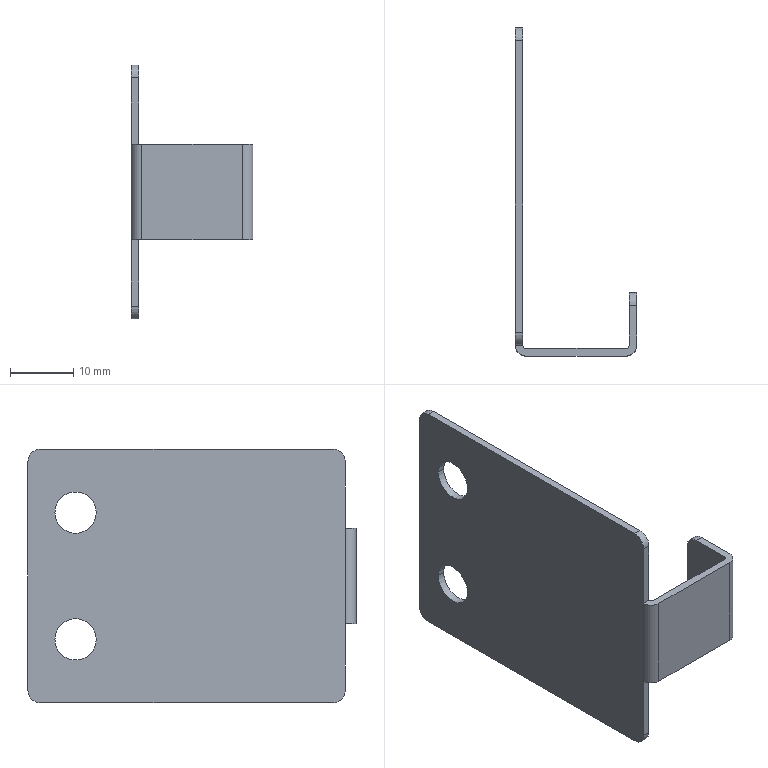Part | SolidWorks | features BaseBody 1 | 1 solid | 28 faces | box 19.2 x 51.7 x 40 mm | volume 2810 mm3 | cylinder 14 | plane 14 | commonest cylinder face diameters 4 x6 6.5 x4 1 x2 3.4 x2
STEP:
#1=CARTESIAN_POINT('',(-1.2,45.75,30.));
#2=VERTEX_POINT('',#1);
#3=CARTESIAN_POINT('',(-1.2,39.25,30.));
#4=VERTEX_POINT('',#3);
#5=CARTESIAN_POINT('',(-1.2,42.5,30.));
#6=DIRECTION('',(-1.,0.,0.));
#7=DIRECTION('',(0.,1.,0.));
#8=AXIS2_PLACEMENT_3D('',#5,#6,#7);
#9=CIRCLE('',#8,3.25);
#10=EDGE_CURVE('',#2,#4,#9,.T.);
#11=ORIENTED_EDGE('',*,*,#10,.T.);
#12=CARTESIAN_POINT('',(0.,39.25,30.));
#13=VERTEX_POINT('',#12);
#14=CARTESIAN_POINT('',(-10.,39.25,30.));
#15=DIRECTION('',(1.,0.,0.));
#16=VECTOR('',#15,1000.);
#17=LINE('',#14,#16);
#18=EDGE_CURVE('',#4,#13,#17,.T.);
#19=ORIENTED_EDGE('',*,*,#18,.T.);
#20=CARTESIAN_POINT('',(0.,45.75,30.));
#21=VERTEX_POINT('',#20);
#22=CARTESIAN_POINT('',(0.,42.5,30.));
#23=DIRECTION('',(-1.,0.,0.));
#24=DIRECTION('',(0.,1.,0.));
#25=AXIS2_PLACEMENT_3D('',#22,#23,#24);
#26=CIRCLE('',#25,3.25);
#27=EDGE_CURVE('',#21,#13,#26,.T.);
#28=ORIENTED_EDGE('',*,*,#27,.F.);
#29=CARTESIAN_POINT('',(-10.,45.75,30.));
#30=DIRECTION('',(1.,0.,0.));
#31=VECTOR('',#30,1000.);
#32=LINE('',#29,#31);
#33=EDGE_CURVE('',#2,#21,#32,.T.);
#34=ORIENTED_EDGE('',*,*,#33,.F.);
#35=EDGE_LOOP('',(#11,#19,#28,#34));
#36=FACE_OUTER_BOUND('',#35,.T.);
#37=CARTESIAN_POINT('',(-10.,42.5,30.));
#38=DIRECTION('',(1.,0.,0.));
#39=DIRECTION('',(0.,1.,0.));
#40=AXIS2_PLACEMENT_3D('',#37,#38,#39);
#41=CYLINDRICAL_SURFACE('',#40,3.25);
#42=ADVANCED_FACE('',(#36),#41,.F.);
#43=CARTESIAN_POINT('',(-1.2,45.75,10.));
#44=VERTEX_POINT('',#43);
#45=CARTESIAN_POINT('',(-1.2,39.25,10.));
#46=VERTEX_POINT('',#45);
#47=CARTESIAN_POINT('',(-1.2,42.5,10.));
#48=DIRECTION('',(-1.,0.,0.));
#49=DIRECTION('',(0.,1.,0.));
#50=AXIS2_PLACEMENT_3D('',#47,#48,#49);
#51=CIRCLE('',#50,3.25);
#52=EDGE_CURVE('',#44,#46,#51,.T.);
#53=ORIENTED_EDGE('',*,*,#52,.T.);
#54=CARTESIAN_POINT('',(0.,39.25,10.));
#55=VERTEX_POINT('',#54);
#56=CARTESIAN_POINT('',(-10.,39.25,10.));
#57=DIRECTION('',(1.,0.,0.));
#58=VECTOR('',#57,1000.);
#59=LINE('',#56,#58);
#60=EDGE_CURVE('',#46,#55,#59,.T.);
#61=ORIENTED_EDGE('',*,*,#60,.T.);
#62=CARTESIAN_POINT('',(0.,45.75,10.));
#63=VERTEX_POINT('',#62);
#64=CARTESIAN_POINT('',(0.,42.5,10.));
#65=DIRECTION('',(-1.,0.,0.));
#66=DIRECTION('',(0.,1.,0.));
#67=AXIS2_PLACEMENT_3D('',#64,#65,#66);
#68=CIRCLE('',#67,3.25);
#69=EDGE_CURVE('',#63,#55,#68,.T.);
#70=ORIENTED_EDGE('',*,*,#69,.F.);
#71=CARTESIAN_POINT('',(-10.,45.75,10.));
#72=DIRECTION('',(1.,0.,0.));
#73=VECTOR('',#72,1000.);
#74=LINE('',#71,#73);
#75=EDGE_CURVE('',#44,#63,#74,.T.);
#76=ORIENTED_EDGE('',*,*,#75,.F.);
#77=EDGE_LOOP('',(#53,#61,#70,#76));
#78=FACE_OUTER_BOUND('',#77,.T.);
#79=CARTESIAN_POINT('',(-10.,42.5,10.));
#80=DIRECTION('',(1.,0.,0.));
#81=DIRECTION('',(0.,1.,0.));
#82=AXIS2_PLACEMENT_3D('',#79,#80,#81);
#83=CYLINDRICAL_SURFACE('',#82,3.25);
#84=ADVANCED_FACE('',(#78),#83,.F.);
#85=CARTESIAN_POINT('',(-1.2,48.,0.));
#86=VERTEX_POINT('',#85);
#87=CARTESIAN_POINT('',(-1.2,50.,2.));
#88=VERTEX_POINT('',#87);
#89=CARTESIAN_POINT('',(-1.2,48.,2.));
#90=DIRECTION('',(1.,0.,0.));
#91=DIRECTION('',(0.,0.,-1.));
#92=AXIS2_PLACEMENT_3D('',#89,#90,#91);
#93=CIRCLE('',#92,2.);
#94=EDGE_CURVE('',#86,#88,#93,.T.);
#95=ORIENTED_EDGE('',*,*,#94,.F.);
#96=CARTESIAN_POINT('',(-1.2,2.,0.));
#97=VERTEX_POINT('',#96);
#98=CARTESIAN_POINT('',(-1.2,50.,0.));
#99=DIRECTION('',(0.,1.,0.));
#100=VECTOR('',#99,1000.);
#101=LINE('',#98,#100);
#102=EDGE_CURVE('',#97,#86,#101,.T.);
#103=ORIENTED_EDGE('',*,*,#102,.F.);
#104=CARTESIAN_POINT('',(-1.2,0.,2.));
#105=VERTEX_POINT('',#104);
#106=CARTESIAN_POINT('',(-1.2,2.,2.));
#107=DIRECTION('',(1.,0.,0.));
#108=DIRECTION('',(0.,0.,1.));
#109=AXIS2_PLACEMENT_3D('',#106,#107,#108);
#110=CIRCLE('',#109,2.);
#111=EDGE_CURVE('',#105,#97,#110,.T.);
#112=ORIENTED_EDGE('',*,*,#111,.F.);
#113=CARTESIAN_POINT('',(-1.2,0.,12.5));
#114=VERTEX_POINT('',#113);
#115=CARTESIAN_POINT('',(-1.2,0.,40.));
#116=DIRECTION('',(0.,0.,-1.));
#117=VECTOR('',#116,1000.);
#118=LINE('',#115,#117);
#119=EDGE_CURVE('',#114,#105,#118,.T.);
#120=ORIENTED_EDGE('',*,*,#119,.F.);
#121=CARTESIAN_POINT('',(-1.2,0.,27.5));
#122=VERTEX_POINT('',#121);
#123=CARTESIAN_POINT('',(-1.2,0.,40.));
#124=DIRECTION('',(0.,0.,-1.));
#125=VECTOR('',#124,1000.);
#126=LINE('',#123,#125);
#127=EDGE_CURVE('',#122,#114,#126,.T.);
#128=ORIENTED_EDGE('',*,*,#127,.F.);
#129=CARTESIAN_POINT('',(-1.2,0.,38.));
#130=VERTEX_POINT('',#129);
#131=CARTESIAN_POINT('',(-1.2,0.,40.));
#132=DIRECTION('',(0.,0.,-1.));
#133=VECTOR('',#132,1000.);
#134=LINE('',#131,#133);
#135=EDGE_CURVE('',#130,#122,#134,.T.);
#136=ORIENTED_EDGE('',*,*,#135,.F.);
#137=CARTESIAN_POINT('',(-1.2,2.,40.));
#138=VERTEX_POINT('',#137);
#139=CARTESIAN_POINT('',(-1.2,2.,38.));
#140=DIRECTION('',(1.,0.,0.));
#141=DIRECTION('',(0.,0.,-1.));
#142=AXIS2_PLACEMENT_3D('',#139,#140,#141);
#143=CIRCLE('',#142,2.);
#144=EDGE_CURVE('',#138,#130,#143,.T.);
#145=ORIENTED_EDGE('',*,*,#144,.F.);
#146=CARTESIAN_POINT('',(-1.2,48.,40.));
#147=VERTEX_POINT('',#146);
#148=CARTESIAN_POINT('',(-1.2,50.,40.));
#149=DIRECTION('',(0.,-1.,0.));
#150=VECTOR('',#149,1000.);
#151=LINE('',#148,#150);
#152=EDGE_CURVE('',#147,#138,#151,.T.);
#153=ORIENTED_EDGE('',*,*,#152,.F.);
#154=CARTESIAN_POINT('',(-1.2,50.,38.));
#155=VERTEX_POINT('',#154);
#156=CARTESIAN_POINT('',(-1.2,48.,38.));
#157=DIRECTION('',(1.,0.,0.));
#158=DIRECTION('',(0.,0.,1.));
#159=AXIS2_PLACEMENT_3D('',#156,#157,#158);
#160=CIRCLE('',#159,2.);
#161=EDGE_CURVE('',#155,#147,#160,.T.);
#162=ORIENTED_EDGE('',*,*,#161,.F.);
#163=CARTESIAN_POINT('',(-1.2,50.,40.));
#164=DIRECTION('',(0.,0.,1.));
#165=VECTOR('',#164,1000.);
#166=LINE('',#163,#165);
#167=EDGE_CURVE('',#88,#155,#166,.T.);
#168=ORIENTED_EDGE('',*,*,#167,.F.);
#169=EDGE_LOOP('',(#95,#103,#112,#120,#128,#136,#145,#153,#162,#168));
#170=FACE_OUTER_BOUND('',#169,.T.);
#171=ORIENTED_EDGE('',*,*,#10,.F.);
#172=CARTESIAN_POINT('',(-1.2,42.5,30.));
#173=DIRECTION('',(-1.,0.,0.));
#174=DIRECTION('',(0.,1.,0.));
#175=AXIS2_PLACEMENT_3D('',#172,#173,#174);
#176=CIRCLE('',#175,3.25);
#177=EDGE_CURVE('',#4,#2,#176,.T.);
#178=ORIENTED_EDGE('',*,*,#177,.F.);
#179=EDGE_LOOP('',(#171,#178));
#180=FACE_BOUND('',#179,.T.);
#181=ORIENTED_EDGE('',*,*,#52,.F.);
#182=CARTESIAN_POINT('',(-1.2,42.5,10.));
#183=DIRECTION('',(-1.,0.,0.));
#184=DIRECTION('',(0.,1.,0.));
#185=AXIS2_PLACEMENT_3D('',#182,#183,#184);
#186=CIRCLE('',#185,3.25);
#187=EDGE_CURVE('',#46,#44,#186,.T.);
#188=ORIENTED_EDGE('',*,*,#187,.F.);
#189=EDGE_LOOP('',(#181,#188));
#190=FACE_BOUND('',#189,.T.);
#191=CARTESIAN_POINT('',(-1.2,50.,40.));
#192=DIRECTION('',(1.,0.,0.));
#193=DIRECTION('',(0.,1.,0.));
#194=AXIS2_PLACEMENT_3D('',#191,#192,#193);
#195=PLANE('',#194);
#196=ADVANCED_FACE('',(#170,#180,#190),#195,.F.);
#197=ORIENTED_EDGE('',*,*,#167,.T.);
#198=CARTESIAN_POINT('',(0.,50.,38.));
#199=VERTEX_POINT('',#198);
#200=CARTESIAN_POINT('',(-1.2,50.,38.));
#201=DIRECTION('',(1.,0.,0.));
#202=VECTOR('',#201,1000.);
#203=LINE('',#200,#202);
#204=EDGE_CURVE('',#155,#199,#203,.T.);
#205=ORIENTED_EDGE('',*,*,#204,.T.);
#206=CARTESIAN_POINT('',(0.,50.,2.));
#207=VERTEX_POINT('',#206);
#208=CARTESIAN_POINT('',(0.,50.,40.));
#209=DIRECTION('',(0.,0.,-1.));
#210=VECTOR('',#209,1000.);
#211=LINE('',#208,#210);
#212=EDGE_CURVE('',#199,#207,#211,.T.);
#213=ORIENTED_EDGE('',*,*,#212,.T.);
#214=CARTESIAN_POINT('',(-1.2,50.,2.));
#215=DIRECTION('',(-1.,0.,0.));
#216=VECTOR('',#215,1000.);
#217=LINE('',#214,#216);
#218=EDGE_CURVE('',#207,#88,#217,.T.);
#219=ORIENTED_EDGE('',*,*,#218,.T.);
#220=EDGE_LOOP('',(#197,#205,#213,#219));
#221=FACE_OUTER_BOUND('',#220,.T.);
#222=CARTESIAN_POINT('',(-1.2,50.,40.));
#223=DIRECTION('',(0.,1.,0.));
#224=DIRECTION('',(0.,0.,1.));
#225=AXIS2_PLACEMENT_3D('',#222,#223,#224);
#226=PLANE('',#225);
#227=ADVANCED_FACE('',(#221),#226,.T.);
#228=CARTESIAN_POINT('',(0.,48.,0.));
#229=VERTEX_POINT('',#228);
#230=CARTESIAN_POINT('',(0.,48.,2.));
#231=DIRECTION('',(-1.,0.,0.));
#232=DIRECTION('',(0.,0.,-1.));
#233=AXIS2_PLACEMENT_3D('',#230,#231,#232);
#234=CIRCLE('',#233,2.);
#235=EDGE_CURVE('',#207,#229,#234,.T.);
#236=ORIENTED_EDGE('',*,*,#235,.T.);
#237=CARTESIAN_POINT('',(0.,48.,0.));
#238=DIRECTION('',(-1.,0.,0.));
#239=VECTOR('',#238,1000.);
#240=LINE('',#237,#239);
#241=EDGE_CURVE('',#229,#86,#240,.T.);
#242=ORIENTED_EDGE('',*,*,#241,.T.);
#243=ORIENTED_EDGE('',*,*,#94,.T.);
#244=ORIENTED_EDGE('',*,*,#218,.F.);
#245=EDGE_LOOP('',(#236,#242,#243,#244));
#246=FACE_OUTER_BOUND('',#245,.T.);
#247=CARTESIAN_POINT('',(0.,48.,2.));
#248=DIRECTION('',(1.,0.,0.));
#249=DIRECTION('',(0.,0.,-1.));
#250=AXIS2_PLACEMENT_3D('',#247,#248,#249);
#251=CYLINDRICAL_SURFACE('',#250,2.);
#252=ADVANCED_FACE('',(#246),#251,.T.);
#253=CARTESIAN_POINT('',(0.,2.,0.));
#254=VERTEX_POINT('',#253);
#255=CARTESIAN_POINT('',(0.,0.,0.));
#256=DIRECTION('',(0.,-1.,0.));
#257=VECTOR('',#256,1000.);
#258=LINE('',#255,#257);
#259=EDGE_CURVE('',#229,#254,#258,.T.);
#260=ORIENTED_EDGE('',*,*,#259,.T.);
#261=CARTESIAN_POINT('',(0.,2.,0.));
#262=DIRECTION('',(-1.,0.,0.));
#263=VECTOR('',#262,1000.);
#264=LINE('',#261,#263);
#265=EDGE_CURVE('',#254,#97,#264,.T.);
#266=ORIENTED_EDGE('',*,*,#265,.T.);
#267=ORIENTED_EDGE('',*,*,#102,.T.);
#268=ORIENTED_EDGE('',*,*,#241,.F.);
#269=EDGE_LOOP('',(#260,#266,#267,#268));
#270=FACE_OUTER_BOUND('',#269,.T.);
#271=CARTESIAN_POINT('',(0.,0.,0.));
#272=DIRECTION('',(0.,0.,-1.));
#273=DIRECTION('',(-1.,0.,0.));
#274=AXIS2_PLACEMENT_3D('',#271,#272,#273);
#275=PLANE('',#274);
#276=ADVANCED_FACE('',(#270),#275,.T.);
#277=ORIENTED_EDGE('',*,*,#111,.T.);
#278=ORIENTED_EDGE('',*,*,#265,.F.);
#279=CARTESIAN_POINT('',(0.,0.,2.));
#280=VERTEX_POINT('',#279);
#281=CARTESIAN_POINT('',(0.,2.,2.));
#282=DIRECTION('',(-1.,0.,0.));
#283=DIRECTION('',(0.,0.,1.));
#284=AXIS2_PLACEMENT_3D('',#281,#282,#283);
#285=CIRCLE('',#284,2.);
#286=EDGE_CURVE('',#254,#280,#285,.T.);
#287=ORIENTED_EDGE('',*,*,#286,.T.);
#288=CARTESIAN_POINT('',(0.,0.,2.));
#289=DIRECTION('',(-1.,0.,0.));
#290=VECTOR('',#289,1000.);
#291=LINE('',#288,#290);
#292=EDGE_CURVE('',#280,#105,#291,.T.);
#293=ORIENTED_EDGE('',*,*,#292,.T.);
#294=EDGE_LOOP('',(#277,#278,#287,#293));
#295=FACE_OUTER_BOUND('',#294,.T.);
#296=CARTESIAN_POINT('',(0.,2.,2.));
#297=DIRECTION('',(-1.,0.,0.));
#298=DIRECTION('',(0.,0.,1.));
#299=AXIS2_PLACEMENT_3D('',#296,#297,#298);
#300=CYLINDRICAL_SURFACE('',#299,2.);
#301=ADVANCED_FACE('',(#295),#300,.T.);
#302=CARTESIAN_POINT('',(0.,0.,12.5));
#303=VERTEX_POINT('',#302);
#304=CARTESIAN_POINT('',(0.,0.,40.));
#305=DIRECTION('',(0.,0.,1.));
#306=VECTOR('',#305,1000.);
#307=LINE('',#304,#306);
#308=EDGE_CURVE('',#280,#303,#307,.T.);
#309=ORIENTED_EDGE('',*,*,#308,.T.);
#310=CARTESIAN_POINT('',(0.5,0.,12.5));
#311=DIRECTION('',(-1.,0.,0.));
#312=VECTOR('',#311,1000.);
#313=LINE('',#310,#312);
#314=EDGE_CURVE('',#303,#114,#313,.T.);
#315=ORIENTED_EDGE('',*,*,#314,.T.);
#316=ORIENTED_EDGE('',*,*,#119,.T.);
#317=ORIENTED_EDGE('',*,*,#292,.F.);
#318=EDGE_LOOP('',(#309,#315,#316,#317));
#319=FACE_OUTER_BOUND('',#318,.T.);
#320=CARTESIAN_POINT('',(0.,0.,40.));
#321=DIRECTION('',(0.,-1.,0.));
#322=DIRECTION('',(0.,0.,-1.));
#323=AXIS2_PLACEMENT_3D('',#320,#321,#322);
#324=PLANE('',#323);
#325=ADVANCED_FACE('',(#319),#324,.T.);
#326=CARTESIAN_POINT('',(0.5,-1.7,12.5));
#327=VERTEX_POINT('',#326);
#328=CARTESIAN_POINT('',(0.5,-1.7,27.5));
#329=VERTEX_POINT('',#328);
#330=CARTESIAN_POINT('',(0.5,-1.7,12.5));
#331=DIRECTION('',(0.,0.,1.));
#332=VECTOR('',#331,1000.);
#333=LINE('',#330,#332);
#334=EDGE_CURVE('',#327,#329,#333,.T.);
#335=ORIENTED_EDGE('',*,*,#334,.T.);
#336=CARTESIAN_POINT('',(0.5,0.,27.5));
#337=DIRECTION('',(0.,0.,-1.));
#338=DIRECTION('',(-1.,0.,0.));
#339=AXIS2_PLACEMENT_3D('',#336,#337,#338);
#340=CIRCLE('',#339,1.7);
#341=EDGE_CURVE('',#329,#122,#340,.T.);
#342=ORIENTED_EDGE('',*,*,#341,.T.);
#343=ORIENTED_EDGE('',*,*,#127,.T.);
#344=CARTESIAN_POINT('',(0.5,0.,12.5));
#345=DIRECTION('',(0.,0.,1.));
#346=DIRECTION('',(-1.,0.,0.));
#347=AXIS2_PLACEMENT_3D('',#344,#345,#346);
#348=CIRCLE('',#347,1.7);
#349=EDGE_CURVE('',#114,#327,#348,.T.);
#350=ORIENTED_EDGE('',*,*,#349,.T.);
#351=EDGE_LOOP('',(#335,#342,#343,#350));
#352=FACE_OUTER_BOUND('',#351,.T.);
#353=CARTESIAN_POINT('',(0.5,0.,12.5));
#354=DIRECTION('',(0.,0.,-1.));
#355=DIRECTION('',(-1.,0.,0.));
#356=AXIS2_PLACEMENT_3D('',#353,#354,#355);
#357=CYLINDRICAL_SURFACE('',#356,1.7);
#358=ADVANCED_FACE('',(#352),#357,.T.);
#359=ORIENTED_EDGE('',*,*,#135,.T.);
#360=CARTESIAN_POINT('',(0.,0.,27.5));
#361=VERTEX_POINT('',#360);
#362=CARTESIAN_POINT('',(0.,0.,27.5));
#363=DIRECTION('',(1.,0.,0.));
#364=VECTOR('',#363,1000.);
#365=LINE('',#362,#364);
#366=EDGE_CURVE('',#122,#361,#365,.T.);
#367=ORIENTED_EDGE('',*,*,#366,.T.);
#368=CARTESIAN_POINT('',(0.,0.,38.));
#369=VERTEX_POINT('',#368);
#370=CARTESIAN_POINT('',(0.,0.,40.));
#371=DIRECTION('',(0.,0.,1.));
#372=VECTOR('',#371,1000.);
#373=LINE('',#370,#372);
#374=EDGE_CURVE('',#361,#369,#373,.T.);
#375=ORIENTED_EDGE('',*,*,#374,.T.);
#376=CARTESIAN_POINT('',(0.,0.,38.));
#377=DIRECTION('',(-1.,0.,0.));
#378=VECTOR('',#377,1000.);
#379=LINE('',#376,#378);
#380=EDGE_CURVE('',#369,#130,#379,.T.);
#381=ORIENTED_EDGE('',*,*,#380,.T.);
#382=EDGE_LOOP('',(#359,#367,#375,#381));
#383=FACE_OUTER_BOUND('',#382,.T.);
#384=CARTESIAN_POINT('',(0.,0.,40.));
#385=DIRECTION('',(0.,-1.,0.));
#386=DIRECTION('',(0.,0.,-1.));
#387=AXIS2_PLACEMENT_3D('',#384,#385,#386);
#388=PLANE('',#387);
#389=ADVANCED_FACE('',(#383),#388,.T.);
#390=ORIENTED_EDGE('',*,*,#144,.T.);
#391=ORIENTED_EDGE('',*,*,#380,.F.);
#392=CARTESIAN_POINT('',(0.,2.,40.));
#393=VERTEX_POINT('',#392);
#394=CARTESIAN_POINT('',(0.,2.,38.));
#395=DIRECTION('',(-1.,0.,0.));
#396=DIRECTION('',(0.,0.,-1.));
#397=AXIS2_PLACEMENT_3D('',#394,#395,#396);
#398=CIRCLE('',#397,2.);
#399=EDGE_CURVE('',#369,#393,#398,.T.);
#400=ORIENTED_EDGE('',*,*,#399,.T.);
#401=CARTESIAN_POINT('',(0.,2.,40.));
#402=DIRECTION('',(-1.,0.,0.));
#403=VECTOR('',#402,1000.);
#404=LINE('',#401,#403);
#405=EDGE_CURVE('',#393,#138,#404,.T.);
#406=ORIENTED_EDGE('',*,*,#405,.T.);
#407=EDGE_LOOP('',(#390,#391,#400,#406));
#408=FACE_OUTER_BOUND('',#407,.T.);
#409=CARTESIAN_POINT('',(0.,2.,38.));
#410=DIRECTION('',(1.,0.,0.));
#411=DIRECTION('',(0.,0.,-1.));
#412=AXIS2_PLACEMENT_3D('',#409,#410,#411);
#413=CYLINDRICAL_SURFACE('',#412,2.);
#414=ADVANCED_FACE('',(#408),#413,.T.);
#415=CARTESIAN_POINT('',(0.,48.,40.));
#416=VERTEX_POINT('',#415);
#417=CARTESIAN_POINT('',(0.,48.,40.));
#418=DIRECTION('',(1.,0.,0.));
#419=VECTOR('',#418,1000.);
#420=LINE('',#417,#419);
#421=EDGE_CURVE('',#147,#416,#420,.T.);
#422=ORIENTED_EDGE('',*,*,#421,.F.);
#423=ORIENTED_EDGE('',*,*,#152,.T.);
#424=ORIENTED_EDGE('',*,*,#405,.F.);
#425=CARTESIAN_POINT('',(0.,0.,40.));
#426=DIRECTION('',(0.,-1.,0.));
#427=VECTOR('',#426,1000.);
#428=LINE('',#425,#427);
#429=EDGE_CURVE('',#416,#393,#428,.T.);
#430=ORIENTED_EDGE('',*,*,#429,.F.);
#431=EDGE_LOOP('',(#422,#423,#424,#430));
#432=FACE_OUTER_BOUND('',#431,.T.);
#433=CARTESIAN_POINT('',(0.,0.,40.));
#434=DIRECTION('',(0.,0.,-1.));
#435=DIRECTION('',(-1.,0.,0.));
#436=AXIS2_PLACEMENT_3D('',#433,#434,#435);
#437=PLANE('',#436);
#438=ADVANCED_FACE('',(#432),#437,.F.);
#439=CARTESIAN_POINT('',(0.,48.,38.));
#440=DIRECTION('',(-1.,0.,0.));
#441=DIRECTION('',(0.,0.,1.));
#442=AXIS2_PLACEMENT_3D('',#439,#440,#441);
#443=CIRCLE('',#442,2.);
#444=EDGE_CURVE('',#416,#199,#443,.T.);
#445=ORIENTED_EDGE('',*,*,#444,.T.);
#446=ORIENTED_EDGE('',*,*,#204,.F.);
#447=ORIENTED_EDGE('',*,*,#161,.T.);
#448=ORIENTED_EDGE('',*,*,#421,.T.);
#449=EDGE_LOOP('',(#445,#446,#447,#448));
#450=FACE_OUTER_BOUND('',#449,.T.);
#451=CARTESIAN_POINT('',(-1.2,48.,38.));
#452=DIRECTION('',(-1.,0.,0.));
#453=DIRECTION('',(0.,0.,1.));
#454=AXIS2_PLACEMENT_3D('',#451,#452,#453);
#455=CYLINDRICAL_SURFACE('',#454,2.);
#456=ADVANCED_FACE('',(#450),#455,.T.);
#457=ORIENTED_EDGE('',*,*,#18,.F.);
#458=ORIENTED_EDGE('',*,*,#177,.T.);
#459=ORIENTED_EDGE('',*,*,#33,.T.);
#460=CARTESIAN_POINT('',(0.,42.5,30.));
#461=DIRECTION('',(-1.,0.,0.));
#462=DIRECTION('',(0.,1.,0.));
#463=AXIS2_PLACEMENT_3D('',#460,#461,#462);
#464=CIRCLE('',#463,3.25);
#465=EDGE_CURVE('',#13,#21,#464,.T.);
#466=ORIENTED_EDGE('',*,*,#465,.F.);
#467=EDGE_LOOP('',(#457,#458,#459,#466));
#468=FACE_OUTER_BOUND('',#467,.T.);
#469=CARTESIAN_POINT('',(-10.,42.5,30.));
#470=DIRECTION('',(1.,0.,0.));
#471=DIRECTION('',(0.,1.,0.));
#472=AXIS2_PLACEMENT_3D('',#469,#470,#471);
#473=CYLINDRICAL_SURFACE('',#472,3.25);
#474=ADVANCED_FACE('',(#468),#473,.F.);
#475=ORIENTED_EDGE('',*,*,#60,.F.);
#476=ORIENTED_EDGE('',*,*,#187,.T.);
#477=ORIENTED_EDGE('',*,*,#75,.T.);
#478=CARTESIAN_POINT('',(0.,42.5,10.));
#479=DIRECTION('',(-1.,0.,0.));
#480=DIRECTION('',(0.,1.,0.));
#481=AXIS2_PLACEMENT_3D('',#478,#479,#480);
#482=CIRCLE('',#481,3.25);
#483=EDGE_CURVE('',#55,#63,#482,.T.);
#484=ORIENTED_EDGE('',*,*,#483,.F.);
#485=EDGE_LOOP('',(#475,#476,#477,#484));
#486=FACE_OUTER_BOUND('',#485,.T.);
#487=CARTESIAN_POINT('',(-10.,42.5,10.));
#488=DIRECTION('',(1.,0.,0.));
#489=DIRECTION('',(0.,1.,0.));
#490=AXIS2_PLACEMENT_3D('',#487,#488,#489);
#491=CYLINDRICAL_SURFACE('',#490,3.25);
#492=ADVANCED_FACE('',(#486),#491,.F.);
#493=ORIENTED_EDGE('',*,*,#308,.F.);
#494=ORIENTED_EDGE('',*,*,#286,.F.);
#495=ORIENTED_EDGE('',*,*,#259,.F.);
#496=ORIENTED_EDGE('',*,*,#235,.F.);
#497=ORIENTED_EDGE('',*,*,#212,.F.);
#498=ORIENTED_EDGE('',*,*,#444,.F.);
#499=ORIENTED_EDGE('',*,*,#429,.T.);
#500=ORIENTED_EDGE('',*,*,#399,.F.);
#501=ORIENTED_EDGE('',*,*,#374,.F.);
#502=CARTESIAN_POINT('',(0.,0.,40.));
#503=DIRECTION('',(0.,0.,-1.));
#504=VECTOR('',#503,1000.);
#505=LINE('',#502,#504);
#506=EDGE_CURVE('',#361,#303,#505,.T.);
#507=ORIENTED_EDGE('',*,*,#506,.T.);
#508=EDGE_LOOP('',(#493,#494,#495,#496,#497,#498,#499,#500,#501,#507));
#509=FACE_OUTER_BOUND('',#508,.T.);
#510=ORIENTED_EDGE('',*,*,#27,.T.);
#511=ORIENTED_EDGE('',*,*,#465,.T.);
#512=EDGE_LOOP('',(#510,#511));
#513=FACE_BOUND('',#512,.T.);
#514=ORIENTED_EDGE('',*,*,#69,.T.);
#515=ORIENTED_EDGE('',*,*,#483,.T.);
#516=EDGE_LOOP('',(#514,#515));
#517=FACE_BOUND('',#516,.T.);
#518=CARTESIAN_POINT('',(0.,50.,40.));
#519=DIRECTION('',(1.,0.,0.));
#520=DIRECTION('',(0.,1.,0.));
#521=AXIS2_PLACEMENT_3D('',#518,#519,#520);
#522=PLANE('',#521);
#523=ADVANCED_FACE('',(#509,#513,#517),#522,.T.);
#524=ORIENTED_EDGE('',*,*,#366,.F.);
#525=ORIENTED_EDGE('',*,*,#341,.F.);
#526=CARTESIAN_POINT('',(16.3,-1.7,27.5));
#527=VERTEX_POINT('',#526);
#528=CARTESIAN_POINT('',(0.,-1.7,27.5));
#529=DIRECTION('',(1.,0.,0.));
#530=VECTOR('',#529,1000.);
#531=LINE('',#528,#530);
#532=EDGE_CURVE('',#329,#527,#531,.T.);
#533=ORIENTED_EDGE('',*,*,#532,.T.);
#534=CARTESIAN_POINT('',(18.,0.,27.5));
#535=VERTEX_POINT('',#534);
#536=CARTESIAN_POINT('',(16.3,0.,27.5));
#537=DIRECTION('',(0.,0.,-1.));
#538=DIRECTION('',(-1.,0.,0.));
#539=AXIS2_PLACEMENT_3D('',#536,#537,#538);
#540=CIRCLE('',#539,1.7);
#541=EDGE_CURVE('',#535,#527,#540,.T.);
#542=ORIENTED_EDGE('',*,*,#541,.F.);
#543=CARTESIAN_POINT('',(18.,6.3,27.5));
#544=VERTEX_POINT('',#543);
#545=CARTESIAN_POINT('',(18.,0.,27.5));
#546=DIRECTION('',(0.,1.,0.));
#547=VECTOR('',#546,1000.);
#548=LINE('',#545,#547);
#549=EDGE_CURVE('',#535,#544,#548,.T.);
#550=ORIENTED_EDGE('',*,*,#549,.T.);
#551=CARTESIAN_POINT('',(16.8,6.3,27.5));
#552=VERTEX_POINT('',#551);
#553=CARTESIAN_POINT('',(18.,6.3,27.5));
#554=DIRECTION('',(1.,0.,0.));
#555=VECTOR('',#554,1000.);
#556=LINE('',#553,#555);
#557=EDGE_CURVE('',#552,#544,#556,.T.);
#558=ORIENTED_EDGE('',*,*,#557,.F.);
#559=CARTESIAN_POINT('',(16.8,0.,27.5));
#560=VERTEX_POINT('',#559);
#561=CARTESIAN_POINT('',(16.8,-0.5,27.5));
#562=DIRECTION('',(0.,1.,0.));
#563=VECTOR('',#562,1000.);
#564=LINE('',#561,#563);
#565=EDGE_CURVE('',#560,#552,#564,.T.);
#566=ORIENTED_EDGE('',*,*,#565,.F.);
#567=CARTESIAN_POINT('',(16.3,-0.5,27.5));
#568=VERTEX_POINT('',#567);
#569=CARTESIAN_POINT('',(16.3,0.,27.5));
#570=DIRECTION('',(0.,0.,-1.));
#571=DIRECTION('',(-1.,0.,0.));
#572=AXIS2_PLACEMENT_3D('',#569,#570,#571);
#573=CIRCLE('',#572,0.5);
#574=EDGE_CURVE('',#560,#568,#573,.T.);
#575=ORIENTED_EDGE('',*,*,#574,.T.);
#576=CARTESIAN_POINT('',(0.5,-0.5,27.5));
#577=VERTEX_POINT('',#576);
#578=CARTESIAN_POINT('',(0.,-0.5,27.5));
#579=DIRECTION('',(1.,0.,0.));
#580=VECTOR('',#579,1000.);
#581=LINE('',#578,#580);
#582=EDGE_CURVE('',#577,#568,#581,.T.);
#583=ORIENTED_EDGE('',*,*,#582,.F.);
#584=CARTESIAN_POINT('',(0.5,0.,27.5));
#585=DIRECTION('',(0.,0.,-1.));
#586=DIRECTION('',(-1.,0.,0.));
#587=AXIS2_PLACEMENT_3D('',#584,#585,#586);
#588=CIRCLE('',#587,0.5);
#589=EDGE_CURVE('',#577,#361,#588,.T.);
#590=ORIENTED_EDGE('',*,*,#589,.T.);
#591=EDGE_LOOP('',(#524,#525,#533,#542,#550,#558,#566,#575,#583,#590));
#592=FACE_OUTER_BOUND('',#591,.T.);
#593=CARTESIAN_POINT('',(0.5,0.,27.5));
#594=DIRECTION('',(0.,0.,1.));
#595=DIRECTION('',(1.,0.,0.));
#596=AXIS2_PLACEMENT_3D('',#593,#594,#595);
#597=PLANE('',#596);
#598=ADVANCED_FACE('',(#592),#597,.T.);
#599=ORIENTED_EDGE('',*,*,#532,.F.);
#600=ORIENTED_EDGE('',*,*,#334,.F.);
#601=CARTESIAN_POINT('',(16.3,-1.7,12.5));
#602=VERTEX_POINT('',#601);
#603=CARTESIAN_POINT('',(0.,-1.7,12.5));
#604=DIRECTION('',(-1.,0.,0.));
#605=VECTOR('',#604,1000.);
#606=LINE('',#603,#605);
#607=EDGE_CURVE('',#602,#327,#606,.T.);
#608=ORIENTED_EDGE('',*,*,#607,.F.);
#609=CARTESIAN_POINT('',(16.3,-1.7,0.));
#610=DIRECTION('',(0.,0.,-1.));
#611=VECTOR('',#610,1000.);
#612=LINE('',#609,#611);
#613=EDGE_CURVE('',#527,#602,#612,.T.);
#614=ORIENTED_EDGE('',*,*,#613,.F.);
#615=EDGE_LOOP('',(#599,#600,#608,#614));
#616=FACE_OUTER_BOUND('',#615,.T.);
#617=CARTESIAN_POINT('',(0.,-1.7,0.));
#618=DIRECTION('',(0.,1.,0.));
#619=DIRECTION('',(-1.,0.,0.));
#620=AXIS2_PLACEMENT_3D('',#617,#618,#619);
#621=PLANE('',#620);
#622=ADVANCED_FACE('',(#616),#621,.F.);
#623=CARTESIAN_POINT('',(0.5,-0.5,12.5));
#624=VERTEX_POINT('',#623);
#625=CARTESIAN_POINT('',(0.5,0.,12.5));
#626=DIRECTION('',(0.,0.,-1.));
#627=DIRECTION('',(-1.,0.,0.));
#628=AXIS2_PLACEMENT_3D('',#625,#626,#627);
#629=CIRCLE('',#628,0.5);
#630=EDGE_CURVE('',#624,#303,#629,.T.);
#631=ORIENTED_EDGE('',*,*,#630,.F.);
#632=CARTESIAN_POINT('',(16.3,-0.5,12.5));
#633=VERTEX_POINT('',#632);
#634=CARTESIAN_POINT('',(18.,-0.5,12.5));
#635=DIRECTION('',(-1.,0.,0.));
#636=VECTOR('',#635,1000.);
#637=LINE('',#634,#636);
#638=EDGE_CURVE('',#633,#624,#637,.T.);
#639=ORIENTED_EDGE('',*,*,#638,.F.);
#640=CARTESIAN_POINT('',(16.8,0.,12.5));
#641=VERTEX_POINT('',#640);
#642=CARTESIAN_POINT('',(16.3,0.,12.5));
#643=DIRECTION('',(0.,0.,-1.));
#644=DIRECTION('',(-1.,0.,0.));
#645=AXIS2_PLACEMENT_3D('',#642,#643,#644);
#646=CIRCLE('',#645,0.5);
#647=EDGE_CURVE('',#641,#633,#646,.T.);
#648=ORIENTED_EDGE('',*,*,#647,.F.);
#649=CARTESIAN_POINT('',(16.8,6.3,12.5));
#650=VERTEX_POINT('',#649);
#651=CARTESIAN_POINT('',(16.8,8.3,12.5));
#652=DIRECTION('',(0.,-1.,0.));
#653=VECTOR('',#652,1000.);
#654=LINE('',#651,#653);
#655=EDGE_CURVE('',#650,#641,#654,.T.);
#656=ORIENTED_EDGE('',*,*,#655,.F.);
#657=CARTESIAN_POINT('',(18.,6.3,12.5));
#658=VERTEX_POINT('',#657);
#659=CARTESIAN_POINT('',(18.,6.3,12.5));
#660=DIRECTION('',(-1.,0.,0.));
#661=VECTOR('',#660,1000.);
#662=LINE('',#659,#661);
#663=EDGE_CURVE('',#658,#650,#662,.T.);
#664=ORIENTED_EDGE('',*,*,#663,.F.);
#665=CARTESIAN_POINT('',(18.,0.,12.5));
#666=VERTEX_POINT('',#665);
#667=CARTESIAN_POINT('',(18.,0.,12.5));
#668=DIRECTION('',(0.,-1.,0.));
#669=VECTOR('',#668,1000.);
#670=LINE('',#667,#669);
#671=EDGE_CURVE('',#658,#666,#670,.T.);
#672=ORIENTED_EDGE('',*,*,#671,.T.);
#673=CARTESIAN_POINT('',(16.3,0.,12.5));
#674=DIRECTION('',(0.,0.,1.));
#675=DIRECTION('',(-1.,0.,0.));
#676=AXIS2_PLACEMENT_3D('',#673,#674,#675);
#677=CIRCLE('',#676,1.7);
#678=EDGE_CURVE('',#602,#666,#677,.T.);
#679=ORIENTED_EDGE('',*,*,#678,.F.);
#680=ORIENTED_EDGE('',*,*,#607,.T.);
#681=ORIENTED_EDGE('',*,*,#349,.F.);
#682=ORIENTED_EDGE('',*,*,#314,.F.);
#683=EDGE_LOOP('',(#631,#639,#648,#656,#664,#672,#679,#680,#681,#682));
#684=FACE_OUTER_BOUND('',#683,.T.);
#685=CARTESIAN_POINT('',(0.5,0.,12.5));
#686=DIRECTION('',(0.,0.,1.));
#687=DIRECTION('',(1.,0.,0.));
#688=AXIS2_PLACEMENT_3D('',#685,#686,#687);
#689=PLANE('',#688);
#690=ADVANCED_FACE('',(#684),#689,.F.);
#691=ORIENTED_EDGE('',*,*,#589,.F.);
#692=CARTESIAN_POINT('',(0.5,-0.5,12.5));
#693=DIRECTION('',(0.,0.,1.));
#694=VECTOR('',#693,1000.);
#695=LINE('',#692,#694);
#696=EDGE_CURVE('',#624,#577,#695,.T.);
#697=ORIENTED_EDGE('',*,*,#696,.F.);
#698=ORIENTED_EDGE('',*,*,#630,.T.);
#699=ORIENTED_EDGE('',*,*,#506,.F.);
#700=EDGE_LOOP('',(#691,#697,#698,#699));
#701=FACE_OUTER_BOUND('',#700,.T.);
#702=CARTESIAN_POINT('',(0.5,0.,12.5));
#703=DIRECTION('',(0.,0.,-1.));
#704=DIRECTION('',(-1.,0.,0.));
#705=AXIS2_PLACEMENT_3D('',#702,#703,#704);
#706=CYLINDRICAL_SURFACE('',#705,0.5);
#707=ADVANCED_FACE('',(#701),#706,.F.);
#708=CARTESIAN_POINT('',(18.,0.,12.5));
#709=DIRECTION('',(0.,0.,1.));
#710=VECTOR('',#709,1000.);
#711=LINE('',#708,#710);
#712=EDGE_CURVE('',#666,#535,#711,.T.);
#713=ORIENTED_EDGE('',*,*,#712,.T.);
#714=ORIENTED_EDGE('',*,*,#541,.T.);
#715=ORIENTED_EDGE('',*,*,#613,.T.);
#716=ORIENTED_EDGE('',*,*,#678,.T.);
#717=EDGE_LOOP('',(#713,#714,#715,#716));
#718=FACE_OUTER_BOUND('',#717,.T.);
#719=CARTESIAN_POINT('',(16.3,0.,12.5));
#720=DIRECTION('',(0.,0.,-1.));
#721=DIRECTION('',(-1.,0.,0.));
#722=AXIS2_PLACEMENT_3D('',#719,#720,#721);
#723=CYLINDRICAL_SURFACE('',#722,1.7);
#724=ADVANCED_FACE('',(#718),#723,.T.);
#725=ORIENTED_EDGE('',*,*,#638,.T.);
#726=ORIENTED_EDGE('',*,*,#696,.T.);
#727=ORIENTED_EDGE('',*,*,#582,.T.);
#728=CARTESIAN_POINT('',(16.3,-0.5,0.));
#729=DIRECTION('',(0.,0.,-1.));
#730=VECTOR('',#729,1000.);
#731=LINE('',#728,#730);
#732=EDGE_CURVE('',#568,#633,#731,.T.);
#733=ORIENTED_EDGE('',*,*,#732,.T.);
#734=EDGE_LOOP('',(#725,#726,#727,#733));
#735=FACE_OUTER_BOUND('',#734,.T.);
#736=CARTESIAN_POINT('',(0.,-0.5,0.));
#737=DIRECTION('',(0.,1.,0.));
#738=DIRECTION('',(-1.,0.,0.));
#739=AXIS2_PLACEMENT_3D('',#736,#737,#738);
#740=PLANE('',#739);
#741=ADVANCED_FACE('',(#735),#740,.T.);
#742=CARTESIAN_POINT('',(18.,8.3,25.5));
#743=VERTEX_POINT('',#742);
#744=CARTESIAN_POINT('',(18.,6.3,25.5));
#745=DIRECTION('',(-1.,0.,0.));
#746=DIRECTION('',(0.,-1.,0.));
#747=AXIS2_PLACEMENT_3D('',#744,#745,#746);
#748=CIRCLE('',#747,2.);
#749=EDGE_CURVE('',#544,#743,#748,.T.);
#750=ORIENTED_EDGE('',*,*,#749,.F.);
#751=ORIENTED_EDGE('',*,*,#549,.F.);
#752=ORIENTED_EDGE('',*,*,#712,.F.);
#753=ORIENTED_EDGE('',*,*,#671,.F.);
#754=CARTESIAN_POINT('',(18.,8.3,14.5));
#755=VERTEX_POINT('',#754);
#756=CARTESIAN_POINT('',(18.,6.3,14.5));
#757=DIRECTION('',(-1.,0.,0.));
#758=DIRECTION('',(0.,-1.,0.));
#759=AXIS2_PLACEMENT_3D('',#756,#757,#758);
#760=CIRCLE('',#759,2.);
#761=EDGE_CURVE('',#755,#658,#760,.T.);
#762=ORIENTED_EDGE('',*,*,#761,.F.);
#763=CARTESIAN_POINT('',(18.,8.3,0.));
#764=DIRECTION('',(0.,0.,-1.));
#765=VECTOR('',#764,1000.);
#766=LINE('',#763,#765);
#767=EDGE_CURVE('',#743,#755,#766,.T.);
#768=ORIENTED_EDGE('',*,*,#767,.F.);
#769=EDGE_LOOP('',(#750,#751,#752,#753,#762,#768));
#770=FACE_OUTER_BOUND('',#769,.T.);
#771=CARTESIAN_POINT('',(18.,0.,0.));
#772=DIRECTION('',(-1.,0.,0.));
#773=DIRECTION('',(0.,-1.,0.));
#774=AXIS2_PLACEMENT_3D('',#771,#772,#773);
#775=PLANE('',#774);
#776=ADVANCED_FACE('',(#770),#775,.F.);
#777=ORIENTED_EDGE('',*,*,#574,.F.);
#778=CARTESIAN_POINT('',(16.8,0.,12.5));
#779=DIRECTION('',(0.,0.,1.));
#780=VECTOR('',#779,1000.);
#781=LINE('',#778,#780);
#782=EDGE_CURVE('',#641,#560,#781,.T.);
#783=ORIENTED_EDGE('',*,*,#782,.F.);
#784=ORIENTED_EDGE('',*,*,#647,.T.);
#785=ORIENTED_EDGE('',*,*,#732,.F.);
#786=EDGE_LOOP('',(#777,#783,#784,#785));
#787=FACE_OUTER_BOUND('',#786,.T.);
#788=CARTESIAN_POINT('',(16.3,0.,12.5));
#789=DIRECTION('',(0.,0.,-1.));
#790=DIRECTION('',(-1.,0.,0.));
#791=AXIS2_PLACEMENT_3D('',#788,#789,#790);
#792=CYLINDRICAL_SURFACE('',#791,0.5);
#793=ADVANCED_FACE('',(#787),#792,.F.);
#794=CARTESIAN_POINT('',(16.8,8.3,25.5));
#795=VERTEX_POINT('',#794);
#796=CARTESIAN_POINT('',(18.,8.3,25.5));
#797=DIRECTION('',(-1.,0.,0.));
#798=VECTOR('',#797,1000.);
#799=LINE('',#796,#798);
#800=EDGE_CURVE('',#743,#795,#799,.T.);
#801=ORIENTED_EDGE('',*,*,#800,.F.);
#802=ORIENTED_EDGE('',*,*,#767,.T.);
#803=CARTESIAN_POINT('',(16.8,8.3,14.5));
#804=VERTEX_POINT('',#803);
#805=CARTESIAN_POINT('',(18.,8.3,14.5));
#806=DIRECTION('',(1.,0.,0.));
#807=VECTOR('',#806,1000.);
#808=LINE('',#805,#807);
#809=EDGE_CURVE('',#804,#755,#808,.T.);
#810=ORIENTED_EDGE('',*,*,#809,.F.);
#811=CARTESIAN_POINT('',(16.8,8.3,27.5));
#812=DIRECTION('',(0.,0.,-1.));
#813=VECTOR('',#812,1000.);
#814=LINE('',#811,#813);
#815=EDGE_CURVE('',#795,#804,#814,.T.);
#816=ORIENTED_EDGE('',*,*,#815,.F.);
#817=EDGE_LOOP('',(#801,#802,#810,#816));
#818=FACE_OUTER_BOUND('',#817,.T.);
#819=CARTESIAN_POINT('',(18.,8.3,27.5));
#820=DIRECTION('',(0.,-1.,0.));
#821=DIRECTION('',(1.,0.,0.));
#822=AXIS2_PLACEMENT_3D('',#819,#820,#821);
#823=PLANE('',#822);
#824=ADVANCED_FACE('',(#818),#823,.F.);
#825=CARTESIAN_POINT('',(16.8,6.3,25.5));
#826=DIRECTION('',(1.,0.,0.));
#827=DIRECTION('',(0.,-1.,0.));
#828=AXIS2_PLACEMENT_3D('',#825,#826,#827);
#829=CIRCLE('',#828,2.);
#830=EDGE_CURVE('',#795,#552,#829,.T.);
#831=ORIENTED_EDGE('',*,*,#830,.T.);
#832=ORIENTED_EDGE('',*,*,#557,.T.);
#833=ORIENTED_EDGE('',*,*,#749,.T.);
#834=ORIENTED_EDGE('',*,*,#800,.T.);
#835=EDGE_LOOP('',(#831,#832,#833,#834));
#836=FACE_OUTER_BOUND('',#835,.T.);
#837=CARTESIAN_POINT('',(18.,6.3,25.5));
#838=DIRECTION('',(-1.,0.,0.));
#839=DIRECTION('',(0.,-1.,0.));
#840=AXIS2_PLACEMENT_3D('',#837,#838,#839);
#841=CYLINDRICAL_SURFACE('',#840,2.);
#842=ADVANCED_FACE('',(#836),#841,.T.);
#843=CARTESIAN_POINT('',(16.8,6.3,14.5));
#844=DIRECTION('',(1.,0.,0.));
#845=DIRECTION('',(0.,-1.,0.));
#846=AXIS2_PLACEMENT_3D('',#843,#844,#845);
#847=CIRCLE('',#846,2.);
#848=EDGE_CURVE('',#650,#804,#847,.T.);
#849=ORIENTED_EDGE('',*,*,#848,.T.);
#850=ORIENTED_EDGE('',*,*,#809,.T.);
#851=ORIENTED_EDGE('',*,*,#761,.T.);
#852=ORIENTED_EDGE('',*,*,#663,.T.);
#853=EDGE_LOOP('',(#849,#850,#851,#852));
#854=FACE_OUTER_BOUND('',#853,.T.);
#855=CARTESIAN_POINT('',(18.,6.3,14.5));
#856=DIRECTION('',(-1.,0.,0.));
#857=DIRECTION('',(0.,-1.,0.));
#858=AXIS2_PLACEMENT_3D('',#855,#856,#857);
#859=CYLINDRICAL_SURFACE('',#858,2.);
#860=ADVANCED_FACE('',(#854),#859,.T.);
#861=ORIENTED_EDGE('',*,*,#655,.T.);
#862=ORIENTED_EDGE('',*,*,#782,.T.);
#863=ORIENTED_EDGE('',*,*,#565,.T.);
#864=ORIENTED_EDGE('',*,*,#830,.F.);
#865=ORIENTED_EDGE('',*,*,#815,.T.);
#866=ORIENTED_EDGE('',*,*,#848,.F.);
#867=EDGE_LOOP('',(#861,#862,#863,#864,#865,#866));
#868=FACE_OUTER_BOUND('',#867,.T.);
#869=CARTESIAN_POINT('',(16.8,0.,0.));
#870=DIRECTION('',(-1.,0.,0.));
#871=DIRECTION('',(0.,-1.,0.));
#872=AXIS2_PLACEMENT_3D('',#869,#870,#871);
#873=PLANE('',#872);
#874=ADVANCED_FACE('',(#868),#873,.T.);
#875=CLOSED_SHELL('',(#42,#84,#196,#227,#252,#276,#301,#325,#358,#389,#414,#438,#456,#474,#492,#523,#598,#622,#690,#707,#724,#741,#776,#793,#824,#842,#860,#874));
#876=MANIFOLD_SOLID_BREP('',#875);
#877=CARTESIAN_POINT('',(0.,0.,0.));
#878=DIRECTION('',(0.,0.,1.));
#879=DIRECTION('',(1.,0.,0.));
#880=AXIS2_PLACEMENT_3D('',#877,#878,#879);
#881=(LENGTH_UNIT()NAMED_UNIT(*)SI_UNIT(.MILLI.,.METRE.));
#882=UNCERTAINTY_MEASURE_WITH_UNIT(LENGTH_MEASURE(0.00001),#881,'','');
#883=(NAMED_UNIT(*)PLANE_ANGLE_UNIT()SI_UNIT($,.RADIAN.));
#884=(NAMED_UNIT(*)SI_UNIT($,.STERADIAN.)SOLID_ANGLE_UNIT());
#885=(GEOMETRIC_REPRESENTATION_CONTEXT(3)GLOBAL_UNCERTAINTY_ASSIGNED_CONTEXT((#882))GLOBAL_UNIT_ASSIGNED_CONTEXT((#881,#883,#884))REPRESENTATION_CONTEXT('',''));
#886=ADVANCED_BREP_SHAPE_REPRESENTATION('',(#876,#880),#885);